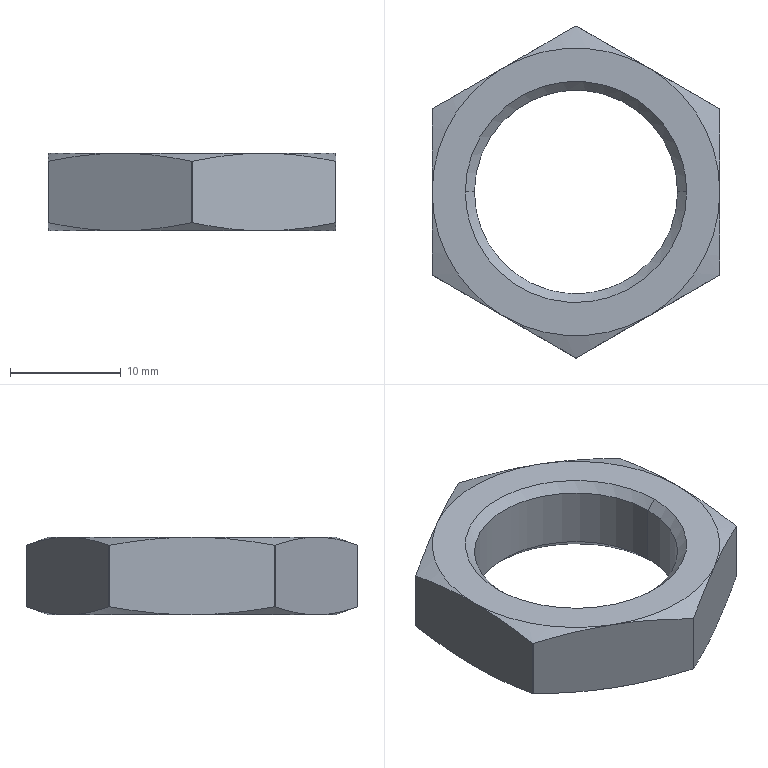Part | SolidWorks | features BaseBody 1 | 1 solid | 32 faces | box 26 x 30 x 7 mm | volume 2178 mm3 | cone 16 | cylinder 8 | plane 8 | commonest cylinder face diameters 30 x6 18.376 x2